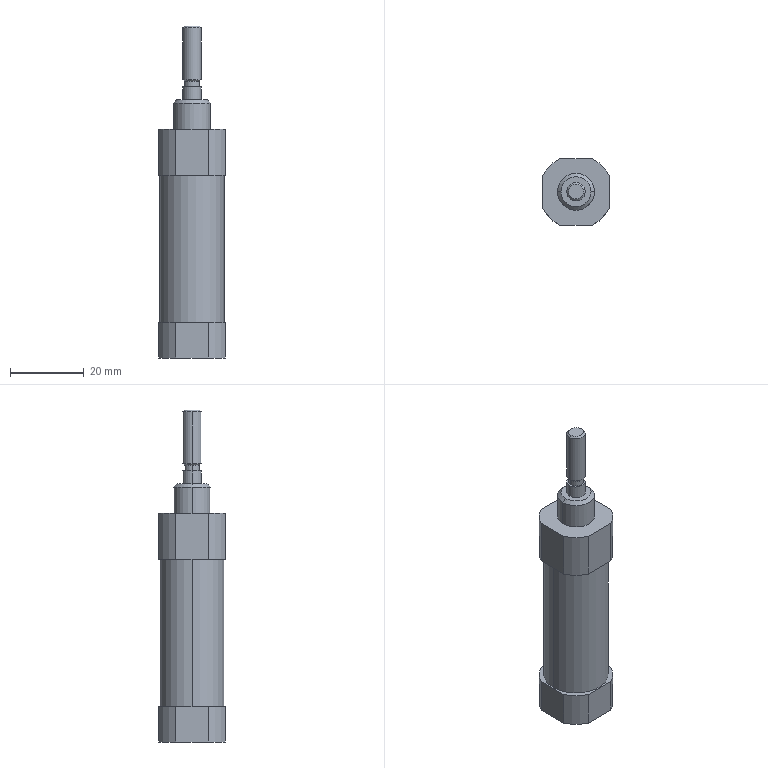Part | STEP file | CDJ2B16-15-B | 1 solid | 49 faces | box 18 x 18 x 90 mm | volume 16817 mm3 | cylinder 22 | plane 17 | cone 10 | commonest cylinder face diameters 20 x8 4.13 x4 5 x4 4.02 x2 10 x2 17.4 x2